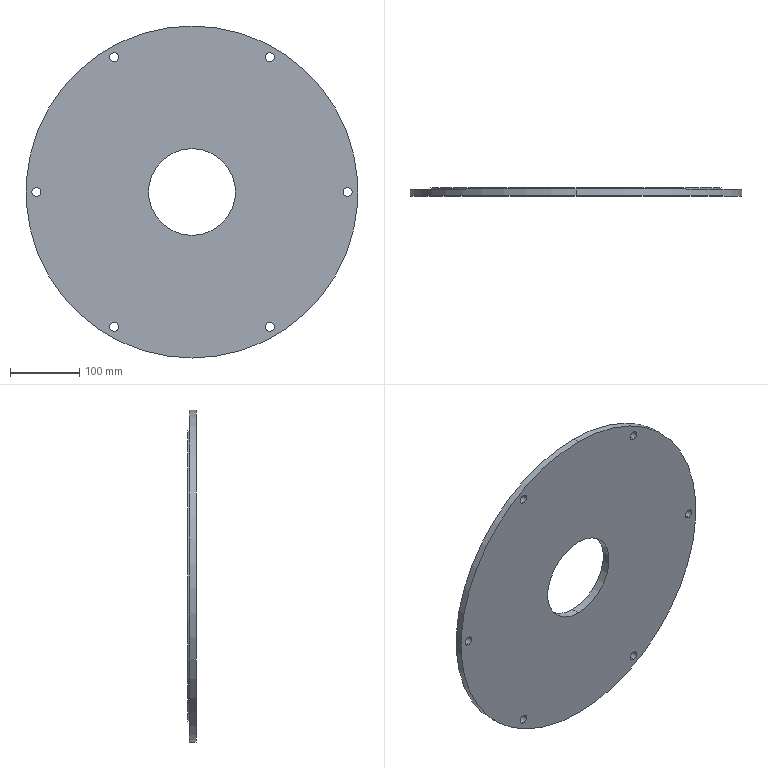Part | SolidWorks | features Extrusion 1, HoleWzd 1, ICE 1 | 1 solid | 21 faces | box 480 x 12 x 480 mm | volume 1930239 mm3 | cylinder 18 | plane 3 | commonest cylinder face diameters 13 x12 125.5 x2 420 x2 480 x2
STEP:
#1=CARTESIAN_POINT('',(0.,4.,210.));
#2=VERTEX_POINT('',#1);
#3=CARTESIAN_POINT('',(0.,4.,-210.));
#4=VERTEX_POINT('',#3);
#5=CARTESIAN_POINT('',(0.,4.,0.));
#6=DIRECTION('',(0.,1.,0.));
#7=DIRECTION('',(0.,0.,1.));
#8=AXIS2_PLACEMENT_3D('',#5,#6,#7);
#9=CIRCLE('',#8,210.);
#10=EDGE_CURVE('',#2,#4,#9,.T.);
#11=ORIENTED_EDGE('',*,*,#10,.T.);
#12=CARTESIAN_POINT('',(0.,6.,-210.));
#13=VERTEX_POINT('',#12);
#14=CARTESIAN_POINT('',(0.,4.,-210.));
#15=DIRECTION('',(0.,1.,0.));
#16=VECTOR('',#15,1000.);
#17=LINE('',#14,#16);
#18=EDGE_CURVE('',#4,#13,#17,.T.);
#19=ORIENTED_EDGE('',*,*,#18,.T.);
#20=CARTESIAN_POINT('',(0.,6.,210.));
#21=VERTEX_POINT('',#20);
#22=CARTESIAN_POINT('',(0.,6.,0.));
#23=DIRECTION('',(0.,1.,0.));
#24=DIRECTION('',(0.,0.,1.));
#25=AXIS2_PLACEMENT_3D('',#22,#23,#24);
#26=CIRCLE('',#25,210.);
#27=EDGE_CURVE('',#21,#13,#26,.T.);
#28=ORIENTED_EDGE('',*,*,#27,.F.);
#29=CARTESIAN_POINT('',(0.,4.,210.));
#30=DIRECTION('',(0.,1.,0.));
#31=VECTOR('',#30,1000.);
#32=LINE('',#29,#31);
#33=EDGE_CURVE('',#2,#21,#32,.T.);
#34=ORIENTED_EDGE('',*,*,#33,.F.);
#35=EDGE_LOOP('',(#11,#19,#28,#34));
#36=FACE_OUTER_BOUND('',#35,.T.);
#37=CARTESIAN_POINT('',(0.,4.,0.));
#38=DIRECTION('',(0.,1.,0.));
#39=DIRECTION('',(0.,0.,1.));
#40=AXIS2_PLACEMENT_3D('',#37,#38,#39);
#41=CYLINDRICAL_SURFACE('',#40,210.);
#42=ADVANCED_FACE('',(#36),#41,.T.);
#43=CARTESIAN_POINT('',(0.,6.,-62.75));
#44=VERTEX_POINT('',#43);
#45=CARTESIAN_POINT('',(0.,6.,62.75));
#46=VERTEX_POINT('',#45);
#47=CARTESIAN_POINT('',(0.,6.,0.));
#48=DIRECTION('',(0.,1.,0.));
#49=DIRECTION('',(0.,0.,1.));
#50=AXIS2_PLACEMENT_3D('',#47,#48,#49);
#51=CIRCLE('',#50,62.75);
#52=EDGE_CURVE('',#44,#46,#51,.T.);
#53=ORIENTED_EDGE('',*,*,#52,.T.);
#54=CARTESIAN_POINT('',(0.,-6.,62.75));
#55=VERTEX_POINT('',#54);
#56=CARTESIAN_POINT('',(0.,6.,62.75));
#57=DIRECTION('',(0.,-1.,0.));
#58=VECTOR('',#57,1000.);
#59=LINE('',#56,#58);
#60=EDGE_CURVE('',#46,#55,#59,.T.);
#61=ORIENTED_EDGE('',*,*,#60,.T.);
#62=CARTESIAN_POINT('',(0.,-6.,-62.75));
#63=VERTEX_POINT('',#62);
#64=CARTESIAN_POINT('',(0.,-6.,0.));
#65=DIRECTION('',(0.,1.,0.));
#66=DIRECTION('',(0.,0.,1.));
#67=AXIS2_PLACEMENT_3D('',#64,#65,#66);
#68=CIRCLE('',#67,62.75);
#69=EDGE_CURVE('',#63,#55,#68,.T.);
#70=ORIENTED_EDGE('',*,*,#69,.F.);
#71=CARTESIAN_POINT('',(0.,6.,-62.75));
#72=DIRECTION('',(0.,-1.,0.));
#73=VECTOR('',#72,1000.);
#74=LINE('',#71,#73);
#75=EDGE_CURVE('',#44,#63,#74,.T.);
#76=ORIENTED_EDGE('',*,*,#75,.F.);
#77=EDGE_LOOP('',(#53,#61,#70,#76));
#78=FACE_OUTER_BOUND('',#77,.T.);
#79=CARTESIAN_POINT('',(0.,6.,0.));
#80=DIRECTION('',(0.,-1.,0.));
#81=DIRECTION('',(0.,0.,-1.));
#82=AXIS2_PLACEMENT_3D('',#79,#80,#81);
#83=CYLINDRICAL_SURFACE('',#82,62.75);
#84=ADVANCED_FACE('',(#78),#83,.F.);
#85=CARTESIAN_POINT('',(112.5,-6.,188.356));
#86=VERTEX_POINT('',#85);
#87=CARTESIAN_POINT('',(112.5,-6.,201.356));
#88=VERTEX_POINT('',#87);
#89=CARTESIAN_POINT('',(112.5,-6.,194.856));
#90=DIRECTION('',(0.,1.,0.));
#91=DIRECTION('',(0.,0.,1.));
#92=AXIS2_PLACEMENT_3D('',#89,#90,#91);
#93=CIRCLE('',#92,6.5);
#94=EDGE_CURVE('',#86,#88,#93,.T.);
#95=ORIENTED_EDGE('',*,*,#94,.F.);
#96=CARTESIAN_POINT('',(112.5,4.,188.356));
#97=VERTEX_POINT('',#96);
#98=CARTESIAN_POINT('',(112.5,6.,188.356));
#99=DIRECTION('',(0.,1.,0.));
#100=VECTOR('',#99,1000.);
#101=LINE('',#98,#100);
#102=EDGE_CURVE('',#86,#97,#101,.T.);
#103=ORIENTED_EDGE('',*,*,#102,.T.);
#104=CARTESIAN_POINT('',(112.5,4.,201.356));
#105=VERTEX_POINT('',#104);
#106=CARTESIAN_POINT('',(112.5,4.,194.856));
#107=DIRECTION('',(0.,-1.,0.));
#108=DIRECTION('',(0.,0.,1.));
#109=AXIS2_PLACEMENT_3D('',#106,#107,#108);
#110=CIRCLE('',#109,6.5);
#111=EDGE_CURVE('',#105,#97,#110,.T.);
#112=ORIENTED_EDGE('',*,*,#111,.F.);
#113=CARTESIAN_POINT('',(112.5,6.,201.356));
#114=DIRECTION('',(0.,1.,0.));
#115=VECTOR('',#114,1000.);
#116=LINE('',#113,#115);
#117=EDGE_CURVE('',#88,#105,#116,.T.);
#118=ORIENTED_EDGE('',*,*,#117,.F.);
#119=EDGE_LOOP('',(#95,#103,#112,#118));
#120=FACE_OUTER_BOUND('',#119,.T.);
#121=CARTESIAN_POINT('',(112.5,6.,194.856));
#122=DIRECTION('',(0.,1.,0.));
#123=DIRECTION('',(0.,0.,1.));
#124=AXIS2_PLACEMENT_3D('',#121,#122,#123);
#125=CYLINDRICAL_SURFACE('',#124,6.5);
#126=ADVANCED_FACE('',(#120),#125,.F.);
#127=CARTESIAN_POINT('',(-112.5,-6.,188.356));
#128=VERTEX_POINT('',#127);
#129=CARTESIAN_POINT('',(-112.5,-6.,201.356));
#130=VERTEX_POINT('',#129);
#131=CARTESIAN_POINT('',(-112.5,-6.,194.856));
#132=DIRECTION('',(0.,1.,0.));
#133=DIRECTION('',(0.,0.,1.));
#134=AXIS2_PLACEMENT_3D('',#131,#132,#133);
#135=CIRCLE('',#134,6.5);
#136=EDGE_CURVE('',#128,#130,#135,.T.);
#137=ORIENTED_EDGE('',*,*,#136,.F.);
#138=CARTESIAN_POINT('',(-112.5,4.,188.356));
#139=VERTEX_POINT('',#138);
#140=CARTESIAN_POINT('',(-112.5,6.,188.356));
#141=DIRECTION('',(0.,1.,0.));
#142=VECTOR('',#141,1000.);
#143=LINE('',#140,#142);
#144=EDGE_CURVE('',#128,#139,#143,.T.);
#145=ORIENTED_EDGE('',*,*,#144,.T.);
#146=CARTESIAN_POINT('',(-112.5,4.,201.356));
#147=VERTEX_POINT('',#146);
#148=CARTESIAN_POINT('',(-112.5,4.,194.856));
#149=DIRECTION('',(0.,-1.,0.));
#150=DIRECTION('',(0.,0.,1.));
#151=AXIS2_PLACEMENT_3D('',#148,#149,#150);
#152=CIRCLE('',#151,6.5);
#153=EDGE_CURVE('',#147,#139,#152,.T.);
#154=ORIENTED_EDGE('',*,*,#153,.F.);
#155=CARTESIAN_POINT('',(-112.5,6.,201.356));
#156=DIRECTION('',(0.,1.,0.));
#157=VECTOR('',#156,1000.);
#158=LINE('',#155,#157);
#159=EDGE_CURVE('',#130,#147,#158,.T.);
#160=ORIENTED_EDGE('',*,*,#159,.F.);
#161=EDGE_LOOP('',(#137,#145,#154,#160));
#162=FACE_OUTER_BOUND('',#161,.T.);
#163=CARTESIAN_POINT('',(-112.5,6.,194.856));
#164=DIRECTION('',(0.,1.,0.));
#165=DIRECTION('',(0.,0.,1.));
#166=AXIS2_PLACEMENT_3D('',#163,#164,#165);
#167=CYLINDRICAL_SURFACE('',#166,6.5);
#168=ADVANCED_FACE('',(#162),#167,.F.);
#169=CARTESIAN_POINT('',(-225.,-6.,-6.5));
#170=VERTEX_POINT('',#169);
#171=CARTESIAN_POINT('',(-225.,-6.,6.5));
#172=VERTEX_POINT('',#171);
#173=CARTESIAN_POINT('',(-225.,-6.,0.));
#174=DIRECTION('',(0.,1.,0.));
#175=DIRECTION('',(0.,0.,1.));
#176=AXIS2_PLACEMENT_3D('',#173,#174,#175);
#177=CIRCLE('',#176,6.5);
#178=EDGE_CURVE('',#170,#172,#177,.T.);
#179=ORIENTED_EDGE('',*,*,#178,.F.);
#180=CARTESIAN_POINT('',(-225.,4.,-6.5));
#181=VERTEX_POINT('',#180);
#182=CARTESIAN_POINT('',(-225.,6.,-6.5));
#183=DIRECTION('',(0.,1.,0.));
#184=VECTOR('',#183,1000.);
#185=LINE('',#182,#184);
#186=EDGE_CURVE('',#170,#181,#185,.T.);
#187=ORIENTED_EDGE('',*,*,#186,.T.);
#188=CARTESIAN_POINT('',(-225.,4.,6.5));
#189=VERTEX_POINT('',#188);
#190=CARTESIAN_POINT('',(-225.,4.,0.));
#191=DIRECTION('',(0.,-1.,0.));
#192=DIRECTION('',(0.,0.,1.));
#193=AXIS2_PLACEMENT_3D('',#190,#191,#192);
#194=CIRCLE('',#193,6.5);
#195=EDGE_CURVE('',#189,#181,#194,.T.);
#196=ORIENTED_EDGE('',*,*,#195,.F.);
#197=CARTESIAN_POINT('',(-225.,6.,6.5));
#198=DIRECTION('',(0.,1.,0.));
#199=VECTOR('',#198,1000.);
#200=LINE('',#197,#199);
#201=EDGE_CURVE('',#172,#189,#200,.T.);
#202=ORIENTED_EDGE('',*,*,#201,.F.);
#203=EDGE_LOOP('',(#179,#187,#196,#202));
#204=FACE_OUTER_BOUND('',#203,.T.);
#205=CARTESIAN_POINT('',(-225.,6.,0.));
#206=DIRECTION('',(0.,1.,0.));
#207=DIRECTION('',(0.,0.,1.));
#208=AXIS2_PLACEMENT_3D('',#205,#206,#207);
#209=CYLINDRICAL_SURFACE('',#208,6.5);
#210=ADVANCED_FACE('',(#204),#209,.F.);
#211=CARTESIAN_POINT('',(-112.5,-6.,-201.356));
#212=VERTEX_POINT('',#211);
#213=CARTESIAN_POINT('',(-112.5,-6.,-188.356));
#214=VERTEX_POINT('',#213);
#215=CARTESIAN_POINT('',(-112.5,-6.,-194.856));
#216=DIRECTION('',(0.,1.,0.));
#217=DIRECTION('',(0.,0.,1.));
#218=AXIS2_PLACEMENT_3D('',#215,#216,#217);
#219=CIRCLE('',#218,6.5);
#220=EDGE_CURVE('',#212,#214,#219,.T.);
#221=ORIENTED_EDGE('',*,*,#220,.F.);
#222=CARTESIAN_POINT('',(-112.5,4.,-201.356));
#223=VERTEX_POINT('',#222);
#224=CARTESIAN_POINT('',(-112.5,6.,-201.356));
#225=DIRECTION('',(0.,1.,0.));
#226=VECTOR('',#225,1000.);
#227=LINE('',#224,#226);
#228=EDGE_CURVE('',#212,#223,#227,.T.);
#229=ORIENTED_EDGE('',*,*,#228,.T.);
#230=CARTESIAN_POINT('',(-112.5,4.,-188.356));
#231=VERTEX_POINT('',#230);
#232=CARTESIAN_POINT('',(-112.5,4.,-194.856));
#233=DIRECTION('',(0.,-1.,0.));
#234=DIRECTION('',(0.,0.,1.));
#235=AXIS2_PLACEMENT_3D('',#232,#233,#234);
#236=CIRCLE('',#235,6.5);
#237=EDGE_CURVE('',#231,#223,#236,.T.);
#238=ORIENTED_EDGE('',*,*,#237,.F.);
#239=CARTESIAN_POINT('',(-112.5,6.,-188.356));
#240=DIRECTION('',(0.,1.,0.));
#241=VECTOR('',#240,1000.);
#242=LINE('',#239,#241);
#243=EDGE_CURVE('',#214,#231,#242,.T.);
#244=ORIENTED_EDGE('',*,*,#243,.F.);
#245=EDGE_LOOP('',(#221,#229,#238,#244));
#246=FACE_OUTER_BOUND('',#245,.T.);
#247=CARTESIAN_POINT('',(-112.5,6.,-194.856));
#248=DIRECTION('',(0.,1.,0.));
#249=DIRECTION('',(0.,0.,1.));
#250=AXIS2_PLACEMENT_3D('',#247,#248,#249);
#251=CYLINDRICAL_SURFACE('',#250,6.5);
#252=ADVANCED_FACE('',(#246),#251,.F.);
#253=CARTESIAN_POINT('',(112.5,-6.,-201.356));
#254=VERTEX_POINT('',#253);
#255=CARTESIAN_POINT('',(112.5,-6.,-188.356));
#256=VERTEX_POINT('',#255);
#257=CARTESIAN_POINT('',(112.5,-6.,-194.856));
#258=DIRECTION('',(0.,1.,0.));
#259=DIRECTION('',(0.,0.,1.));
#260=AXIS2_PLACEMENT_3D('',#257,#258,#259);
#261=CIRCLE('',#260,6.5);
#262=EDGE_CURVE('',#254,#256,#261,.T.);
#263=ORIENTED_EDGE('',*,*,#262,.F.);
#264=CARTESIAN_POINT('',(112.5,4.,-201.356));
#265=VERTEX_POINT('',#264);
#266=CARTESIAN_POINT('',(112.5,6.,-201.356));
#267=DIRECTION('',(0.,1.,0.));
#268=VECTOR('',#267,1000.);
#269=LINE('',#266,#268);
#270=EDGE_CURVE('',#254,#265,#269,.T.);
#271=ORIENTED_EDGE('',*,*,#270,.T.);
#272=CARTESIAN_POINT('',(112.5,4.,-188.356));
#273=VERTEX_POINT('',#272);
#274=CARTESIAN_POINT('',(112.5,4.,-194.856));
#275=DIRECTION('',(0.,-1.,0.));
#276=DIRECTION('',(0.,0.,1.));
#277=AXIS2_PLACEMENT_3D('',#274,#275,#276);
#278=CIRCLE('',#277,6.5);
#279=EDGE_CURVE('',#273,#265,#278,.T.);
#280=ORIENTED_EDGE('',*,*,#279,.F.);
#281=CARTESIAN_POINT('',(112.5,6.,-188.356));
#282=DIRECTION('',(0.,1.,0.));
#283=VECTOR('',#282,1000.);
#284=LINE('',#281,#283);
#285=EDGE_CURVE('',#256,#273,#284,.T.);
#286=ORIENTED_EDGE('',*,*,#285,.F.);
#287=EDGE_LOOP('',(#263,#271,#280,#286));
#288=FACE_OUTER_BOUND('',#287,.T.);
#289=CARTESIAN_POINT('',(112.5,6.,-194.856));
#290=DIRECTION('',(0.,1.,0.));
#291=DIRECTION('',(0.,0.,1.));
#292=AXIS2_PLACEMENT_3D('',#289,#290,#291);
#293=CYLINDRICAL_SURFACE('',#292,6.5);
#294=ADVANCED_FACE('',(#288),#293,.F.);
#295=CARTESIAN_POINT('',(225.,-6.,-6.5));
#296=VERTEX_POINT('',#295);
#297=CARTESIAN_POINT('',(225.,-6.,6.5));
#298=VERTEX_POINT('',#297);
#299=CARTESIAN_POINT('',(225.,-6.,0.));
#300=DIRECTION('',(0.,1.,0.));
#301=DIRECTION('',(0.,0.,1.));
#302=AXIS2_PLACEMENT_3D('',#299,#300,#301);
#303=CIRCLE('',#302,6.5);
#304=EDGE_CURVE('',#296,#298,#303,.T.);
#305=ORIENTED_EDGE('',*,*,#304,.F.);
#306=CARTESIAN_POINT('',(225.,4.,-6.5));
#307=VERTEX_POINT('',#306);
#308=CARTESIAN_POINT('',(225.,6.,-6.5));
#309=DIRECTION('',(0.,1.,0.));
#310=VECTOR('',#309,1000.);
#311=LINE('',#308,#310);
#312=EDGE_CURVE('',#296,#307,#311,.T.);
#313=ORIENTED_EDGE('',*,*,#312,.T.);
#314=CARTESIAN_POINT('',(225.,4.,6.5));
#315=VERTEX_POINT('',#314);
#316=CARTESIAN_POINT('',(225.,4.,0.));
#317=DIRECTION('',(0.,-1.,0.));
#318=DIRECTION('',(0.,0.,1.));
#319=AXIS2_PLACEMENT_3D('',#316,#317,#318);
#320=CIRCLE('',#319,6.5);
#321=EDGE_CURVE('',#315,#307,#320,.T.);
#322=ORIENTED_EDGE('',*,*,#321,.F.);
#323=CARTESIAN_POINT('',(225.,6.,6.5));
#324=DIRECTION('',(0.,1.,0.));
#325=VECTOR('',#324,1000.);
#326=LINE('',#323,#325);
#327=EDGE_CURVE('',#298,#315,#326,.T.);
#328=ORIENTED_EDGE('',*,*,#327,.F.);
#329=EDGE_LOOP('',(#305,#313,#322,#328));
#330=FACE_OUTER_BOUND('',#329,.T.);
#331=CARTESIAN_POINT('',(225.,6.,0.));
#332=DIRECTION('',(0.,1.,0.));
#333=DIRECTION('',(0.,0.,1.));
#334=AXIS2_PLACEMENT_3D('',#331,#332,#333);
#335=CYLINDRICAL_SURFACE('',#334,6.5);
#336=ADVANCED_FACE('',(#330),#335,.F.);
#337=CARTESIAN_POINT('',(0.,4.,240.));
#338=VERTEX_POINT('',#337);
#339=CARTESIAN_POINT('',(0.,4.,-240.));
#340=VERTEX_POINT('',#339);
#341=CARTESIAN_POINT('',(0.,4.,0.));
#342=DIRECTION('',(0.,1.,0.));
#343=DIRECTION('',(0.,0.,1.));
#344=AXIS2_PLACEMENT_3D('',#341,#342,#343);
#345=CIRCLE('',#344,240.);
#346=EDGE_CURVE('',#338,#340,#345,.T.);
#347=ORIENTED_EDGE('',*,*,#346,.F.);
#348=CARTESIAN_POINT('',(0.,-6.,240.));
#349=VERTEX_POINT('',#348);
#350=CARTESIAN_POINT('',(0.,6.,240.));
#351=DIRECTION('',(0.,-1.,0.));
#352=VECTOR('',#351,1000.);
#353=LINE('',#350,#352);
#354=EDGE_CURVE('',#338,#349,#353,.T.);
#355=ORIENTED_EDGE('',*,*,#354,.T.);
#356=CARTESIAN_POINT('',(0.,-6.,-240.));
#357=VERTEX_POINT('',#356);
#358=CARTESIAN_POINT('',(0.,-6.,0.));
#359=DIRECTION('',(0.,1.,0.));
#360=DIRECTION('',(0.,0.,1.));
#361=AXIS2_PLACEMENT_3D('',#358,#359,#360);
#362=CIRCLE('',#361,240.);
#363=EDGE_CURVE('',#349,#357,#362,.T.);
#364=ORIENTED_EDGE('',*,*,#363,.T.);
#365=CARTESIAN_POINT('',(0.,6.,-240.));
#366=DIRECTION('',(0.,-1.,0.));
#367=VECTOR('',#366,1000.);
#368=LINE('',#365,#367);
#369=EDGE_CURVE('',#340,#357,#368,.T.);
#370=ORIENTED_EDGE('',*,*,#369,.F.);
#371=EDGE_LOOP('',(#347,#355,#364,#370));
#372=FACE_OUTER_BOUND('',#371,.T.);
#373=CARTESIAN_POINT('',(0.,6.,0.));
#374=DIRECTION('',(0.,-1.,0.));
#375=DIRECTION('',(0.,0.,-1.));
#376=AXIS2_PLACEMENT_3D('',#373,#374,#375);
#377=CYLINDRICAL_SURFACE('',#376,240.);
#378=ADVANCED_FACE('',(#372),#377,.T.);
#379=ORIENTED_EDGE('',*,*,#52,.F.);
#380=CARTESIAN_POINT('',(0.,6.,0.));
#381=DIRECTION('',(0.,1.,0.));
#382=DIRECTION('',(0.,0.,1.));
#383=AXIS2_PLACEMENT_3D('',#380,#381,#382);
#384=CIRCLE('',#383,62.75);
#385=EDGE_CURVE('',#46,#44,#384,.T.);
#386=ORIENTED_EDGE('',*,*,#385,.F.);
#387=EDGE_LOOP('',(#379,#386));
#388=FACE_BOUND('',#387,.T.);
#389=ORIENTED_EDGE('',*,*,#27,.T.);
#390=CARTESIAN_POINT('',(0.,6.,0.));
#391=DIRECTION('',(0.,1.,0.));
#392=DIRECTION('',(0.,0.,1.));
#393=AXIS2_PLACEMENT_3D('',#390,#391,#392);
#394=CIRCLE('',#393,210.);
#395=EDGE_CURVE('',#13,#21,#394,.T.);
#396=ORIENTED_EDGE('',*,*,#395,.T.);
#397=EDGE_LOOP('',(#389,#396));
#398=FACE_OUTER_BOUND('',#397,.T.);
#399=CARTESIAN_POINT('',(0.,6.,0.));
#400=DIRECTION('',(0.,1.,0.));
#401=DIRECTION('',(0.,0.,1.));
#402=AXIS2_PLACEMENT_3D('',#399,#400,#401);
#403=PLANE('',#402);
#404=ADVANCED_FACE('',(#388,#398),#403,.T.);
#405=ORIENTED_EDGE('',*,*,#354,.F.);
#406=CARTESIAN_POINT('',(0.,4.,0.));
#407=DIRECTION('',(0.,1.,0.));
#408=DIRECTION('',(0.,0.,1.));
#409=AXIS2_PLACEMENT_3D('',#406,#407,#408);
#410=CIRCLE('',#409,240.);
#411=EDGE_CURVE('',#340,#338,#410,.T.);
#412=ORIENTED_EDGE('',*,*,#411,.F.);
#413=ORIENTED_EDGE('',*,*,#369,.T.);
#414=CARTESIAN_POINT('',(0.,-6.,0.));
#415=DIRECTION('',(0.,1.,0.));
#416=DIRECTION('',(0.,0.,1.));
#417=AXIS2_PLACEMENT_3D('',#414,#415,#416);
#418=CIRCLE('',#417,240.);
#419=EDGE_CURVE('',#357,#349,#418,.T.);
#420=ORIENTED_EDGE('',*,*,#419,.T.);
#421=EDGE_LOOP('',(#405,#412,#413,#420));
#422=FACE_OUTER_BOUND('',#421,.T.);
#423=CARTESIAN_POINT('',(0.,6.,0.));
#424=DIRECTION('',(0.,-1.,0.));
#425=DIRECTION('',(0.,0.,-1.));
#426=AXIS2_PLACEMENT_3D('',#423,#424,#425);
#427=CYLINDRICAL_SURFACE('',#426,240.);
#428=ADVANCED_FACE('',(#422),#427,.T.);
#429=ORIENTED_EDGE('',*,*,#312,.F.);
#430=CARTESIAN_POINT('',(225.,-6.,0.));
#431=DIRECTION('',(0.,1.,0.));
#432=DIRECTION('',(0.,0.,1.));
#433=AXIS2_PLACEMENT_3D('',#430,#431,#432);
#434=CIRCLE('',#433,6.5);
#435=EDGE_CURVE('',#298,#296,#434,.T.);
#436=ORIENTED_EDGE('',*,*,#435,.F.);
#437=ORIENTED_EDGE('',*,*,#327,.T.);
#438=CARTESIAN_POINT('',(225.,4.,0.));
#439=DIRECTION('',(0.,-1.,0.));
#440=DIRECTION('',(0.,0.,1.));
#441=AXIS2_PLACEMENT_3D('',#438,#439,#440);
#442=CIRCLE('',#441,6.5);
#443=EDGE_CURVE('',#307,#315,#442,.T.);
#444=ORIENTED_EDGE('',*,*,#443,.F.);
#445=EDGE_LOOP('',(#429,#436,#437,#444));
#446=FACE_OUTER_BOUND('',#445,.T.);
#447=CARTESIAN_POINT('',(225.,6.,0.));
#448=DIRECTION('',(0.,1.,0.));
#449=DIRECTION('',(0.,0.,1.));
#450=AXIS2_PLACEMENT_3D('',#447,#448,#449);
#451=CYLINDRICAL_SURFACE('',#450,6.5);
#452=ADVANCED_FACE('',(#446),#451,.F.);
#453=ORIENTED_EDGE('',*,*,#270,.F.);
#454=CARTESIAN_POINT('',(112.5,-6.,-194.856));
#455=DIRECTION('',(0.,1.,0.));
#456=DIRECTION('',(0.,0.,1.));
#457=AXIS2_PLACEMENT_3D('',#454,#455,#456);
#458=CIRCLE('',#457,6.5);
#459=EDGE_CURVE('',#256,#254,#458,.T.);
#460=ORIENTED_EDGE('',*,*,#459,.F.);
#461=ORIENTED_EDGE('',*,*,#285,.T.);
#462=CARTESIAN_POINT('',(112.5,4.,-194.856));
#463=DIRECTION('',(0.,-1.,0.));
#464=DIRECTION('',(0.,0.,1.));
#465=AXIS2_PLACEMENT_3D('',#462,#463,#464);
#466=CIRCLE('',#465,6.5);
#467=EDGE_CURVE('',#265,#273,#466,.T.);
#468=ORIENTED_EDGE('',*,*,#467,.F.);
#469=EDGE_LOOP('',(#453,#460,#461,#468));
#470=FACE_OUTER_BOUND('',#469,.T.);
#471=CARTESIAN_POINT('',(112.5,6.,-194.856));
#472=DIRECTION('',(0.,1.,0.));
#473=DIRECTION('',(0.,0.,1.));
#474=AXIS2_PLACEMENT_3D('',#471,#472,#473);
#475=CYLINDRICAL_SURFACE('',#474,6.5);
#476=ADVANCED_FACE('',(#470),#475,.F.);
#477=ORIENTED_EDGE('',*,*,#228,.F.);
#478=CARTESIAN_POINT('',(-112.5,-6.,-194.856));
#479=DIRECTION('',(0.,1.,0.));
#480=DIRECTION('',(0.,0.,1.));
#481=AXIS2_PLACEMENT_3D('',#478,#479,#480);
#482=CIRCLE('',#481,6.5);
#483=EDGE_CURVE('',#214,#212,#482,.T.);
#484=ORIENTED_EDGE('',*,*,#483,.F.);
#485=ORIENTED_EDGE('',*,*,#243,.T.);
#486=CARTESIAN_POINT('',(-112.5,4.,-194.856));
#487=DIRECTION('',(0.,-1.,0.));
#488=DIRECTION('',(0.,0.,1.));
#489=AXIS2_PLACEMENT_3D('',#486,#487,#488);
#490=CIRCLE('',#489,6.5);
#491=EDGE_CURVE('',#223,#231,#490,.T.);
#492=ORIENTED_EDGE('',*,*,#491,.F.);
#493=EDGE_LOOP('',(#477,#484,#485,#492));
#494=FACE_OUTER_BOUND('',#493,.T.);
#495=CARTESIAN_POINT('',(-112.5,6.,-194.856));
#496=DIRECTION('',(0.,1.,0.));
#497=DIRECTION('',(0.,0.,1.));
#498=AXIS2_PLACEMENT_3D('',#495,#496,#497);
#499=CYLINDRICAL_SURFACE('',#498,6.5);
#500=ADVANCED_FACE('',(#494),#499,.F.);
#501=ORIENTED_EDGE('',*,*,#186,.F.);
#502=CARTESIAN_POINT('',(-225.,-6.,0.));
#503=DIRECTION('',(0.,1.,0.));
#504=DIRECTION('',(0.,0.,1.));
#505=AXIS2_PLACEMENT_3D('',#502,#503,#504);
#506=CIRCLE('',#505,6.5);
#507=EDGE_CURVE('',#172,#170,#506,.T.);
#508=ORIENTED_EDGE('',*,*,#507,.F.);
#509=ORIENTED_EDGE('',*,*,#201,.T.);
#510=CARTESIAN_POINT('',(-225.,4.,0.));
#511=DIRECTION('',(0.,-1.,0.));
#512=DIRECTION('',(0.,0.,1.));
#513=AXIS2_PLACEMENT_3D('',#510,#511,#512);
#514=CIRCLE('',#513,6.5);
#515=EDGE_CURVE('',#181,#189,#514,.T.);
#516=ORIENTED_EDGE('',*,*,#515,.F.);
#517=EDGE_LOOP('',(#501,#508,#509,#516));
#518=FACE_OUTER_BOUND('',#517,.T.);
#519=CARTESIAN_POINT('',(-225.,6.,0.));
#520=DIRECTION('',(0.,1.,0.));
#521=DIRECTION('',(0.,0.,1.));
#522=AXIS2_PLACEMENT_3D('',#519,#520,#521);
#523=CYLINDRICAL_SURFACE('',#522,6.5);
#524=ADVANCED_FACE('',(#518),#523,.F.);
#525=ORIENTED_EDGE('',*,*,#144,.F.);
#526=CARTESIAN_POINT('',(-112.5,-6.,194.856));
#527=DIRECTION('',(0.,1.,0.));
#528=DIRECTION('',(0.,0.,1.));
#529=AXIS2_PLACEMENT_3D('',#526,#527,#528);
#530=CIRCLE('',#529,6.5);
#531=EDGE_CURVE('',#130,#128,#530,.T.);
#532=ORIENTED_EDGE('',*,*,#531,.F.);
#533=ORIENTED_EDGE('',*,*,#159,.T.);
#534=CARTESIAN_POINT('',(-112.5,4.,194.856));
#535=DIRECTION('',(0.,-1.,0.));
#536=DIRECTION('',(0.,0.,1.));
#537=AXIS2_PLACEMENT_3D('',#534,#535,#536);
#538=CIRCLE('',#537,6.5);
#539=EDGE_CURVE('',#139,#147,#538,.T.);
#540=ORIENTED_EDGE('',*,*,#539,.F.);
#541=EDGE_LOOP('',(#525,#532,#533,#540));
#542=FACE_OUTER_BOUND('',#541,.T.);
#543=CARTESIAN_POINT('',(-112.5,6.,194.856));
#544=DIRECTION('',(0.,1.,0.));
#545=DIRECTION('',(0.,0.,1.));
#546=AXIS2_PLACEMENT_3D('',#543,#544,#545);
#547=CYLINDRICAL_SURFACE('',#546,6.5);
#548=ADVANCED_FACE('',(#542),#547,.F.);
#549=ORIENTED_EDGE('',*,*,#102,.F.);
#550=CARTESIAN_POINT('',(112.5,-6.,194.856));
#551=DIRECTION('',(0.,1.,0.));
#552=DIRECTION('',(0.,0.,1.));
#553=AXIS2_PLACEMENT_3D('',#550,#551,#552);
#554=CIRCLE('',#553,6.5);
#555=EDGE_CURVE('',#88,#86,#554,.T.);
#556=ORIENTED_EDGE('',*,*,#555,.F.);
#557=ORIENTED_EDGE('',*,*,#117,.T.);
#558=CARTESIAN_POINT('',(112.5,4.,194.856));
#559=DIRECTION('',(0.,-1.,0.));
#560=DIRECTION('',(0.,0.,1.));
#561=AXIS2_PLACEMENT_3D('',#558,#559,#560);
#562=CIRCLE('',#561,6.5);
#563=EDGE_CURVE('',#97,#105,#562,.T.);
#564=ORIENTED_EDGE('',*,*,#563,.F.);
#565=EDGE_LOOP('',(#549,#556,#557,#564));
#566=FACE_OUTER_BOUND('',#565,.T.);
#567=CARTESIAN_POINT('',(112.5,6.,194.856));
#568=DIRECTION('',(0.,1.,0.));
#569=DIRECTION('',(0.,0.,1.));
#570=AXIS2_PLACEMENT_3D('',#567,#568,#569);
#571=CYLINDRICAL_SURFACE('',#570,6.5);
#572=ADVANCED_FACE('',(#566),#571,.F.);
#573=ORIENTED_EDGE('',*,*,#555,.T.);
#574=ORIENTED_EDGE('',*,*,#94,.T.);
#575=EDGE_LOOP('',(#573,#574));
#576=FACE_BOUND('',#575,.T.);
#577=ORIENTED_EDGE('',*,*,#531,.T.);
#578=ORIENTED_EDGE('',*,*,#136,.T.);
#579=EDGE_LOOP('',(#577,#578));
#580=FACE_BOUND('',#579,.T.);
#581=ORIENTED_EDGE('',*,*,#507,.T.);
#582=ORIENTED_EDGE('',*,*,#178,.T.);
#583=EDGE_LOOP('',(#581,#582));
#584=FACE_BOUND('',#583,.T.);
#585=ORIENTED_EDGE('',*,*,#483,.T.);
#586=ORIENTED_EDGE('',*,*,#220,.T.);
#587=EDGE_LOOP('',(#585,#586));
#588=FACE_BOUND('',#587,.T.);
#589=ORIENTED_EDGE('',*,*,#459,.T.);
#590=ORIENTED_EDGE('',*,*,#262,.T.);
#591=EDGE_LOOP('',(#589,#590));
#592=FACE_BOUND('',#591,.T.);
#593=ORIENTED_EDGE('',*,*,#435,.T.);
#594=ORIENTED_EDGE('',*,*,#304,.T.);
#595=EDGE_LOOP('',(#593,#594));
#596=FACE_BOUND('',#595,.T.);
#597=ORIENTED_EDGE('',*,*,#419,.F.);
#598=ORIENTED_EDGE('',*,*,#363,.F.);
#599=EDGE_LOOP('',(#597,#598));
#600=FACE_OUTER_BOUND('',#599,.T.);
#601=ORIENTED_EDGE('',*,*,#69,.T.);
#602=CARTESIAN_POINT('',(0.,-6.,0.));
#603=DIRECTION('',(0.,1.,0.));
#604=DIRECTION('',(0.,0.,1.));
#605=AXIS2_PLACEMENT_3D('',#602,#603,#604);
#606=CIRCLE('',#605,62.75);
#607=EDGE_CURVE('',#55,#63,#606,.T.);
#608=ORIENTED_EDGE('',*,*,#607,.T.);
#609=EDGE_LOOP('',(#601,#608));
#610=FACE_BOUND('',#609,.T.);
#611=CARTESIAN_POINT('',(0.,-6.,0.));
#612=DIRECTION('',(0.,1.,0.));
#613=DIRECTION('',(0.,0.,1.));
#614=AXIS2_PLACEMENT_3D('',#611,#612,#613);
#615=PLANE('',#614);
#616=ADVANCED_FACE('',(#576,#580,#584,#588,#592,#596,#600,#610),#615,.F.);
#617=ORIENTED_EDGE('',*,*,#60,.F.);
#618=ORIENTED_EDGE('',*,*,#385,.T.);
#619=ORIENTED_EDGE('',*,*,#75,.T.);
#620=ORIENTED_EDGE('',*,*,#607,.F.);
#621=EDGE_LOOP('',(#617,#618,#619,#620));
#622=FACE_OUTER_BOUND('',#621,.T.);
#623=CARTESIAN_POINT('',(0.,6.,0.));
#624=DIRECTION('',(0.,-1.,0.));
#625=DIRECTION('',(0.,0.,-1.));
#626=AXIS2_PLACEMENT_3D('',#623,#624,#625);
#627=CYLINDRICAL_SURFACE('',#626,62.75);
#628=ADVANCED_FACE('',(#622),#627,.F.);
#629=ORIENTED_EDGE('',*,*,#321,.T.);
#630=ORIENTED_EDGE('',*,*,#443,.T.);
#631=EDGE_LOOP('',(#629,#630));
#632=FACE_BOUND('',#631,.T.);
#633=ORIENTED_EDGE('',*,*,#279,.T.);
#634=ORIENTED_EDGE('',*,*,#467,.T.);
#635=EDGE_LOOP('',(#633,#634));
#636=FACE_BOUND('',#635,.T.);
#637=ORIENTED_EDGE('',*,*,#237,.T.);
#638=ORIENTED_EDGE('',*,*,#491,.T.);
#639=EDGE_LOOP('',(#637,#638));
#640=FACE_BOUND('',#639,.T.);
#641=ORIENTED_EDGE('',*,*,#195,.T.);
#642=ORIENTED_EDGE('',*,*,#515,.T.);
#643=EDGE_LOOP('',(#641,#642));
#644=FACE_BOUND('',#643,.T.);
#645=ORIENTED_EDGE('',*,*,#153,.T.);
#646=ORIENTED_EDGE('',*,*,#539,.T.);
#647=EDGE_LOOP('',(#645,#646));
#648=FACE_BOUND('',#647,.T.);
#649=ORIENTED_EDGE('',*,*,#111,.T.);
#650=ORIENTED_EDGE('',*,*,#563,.T.);
#651=EDGE_LOOP('',(#649,#650));
#652=FACE_BOUND('',#651,.T.);
#653=ORIENTED_EDGE('',*,*,#10,.F.);
#654=CARTESIAN_POINT('',(0.,4.,0.));
#655=DIRECTION('',(0.,1.,0.));
#656=DIRECTION('',(0.,0.,1.));
#657=AXIS2_PLACEMENT_3D('',#654,#655,#656);
#658=CIRCLE('',#657,210.);
#659=EDGE_CURVE('',#4,#2,#658,.T.);
#660=ORIENTED_EDGE('',*,*,#659,.F.);
#661=EDGE_LOOP('',(#653,#660));
#662=FACE_BOUND('',#661,.T.);
#663=ORIENTED_EDGE('',*,*,#411,.T.);
#664=ORIENTED_EDGE('',*,*,#346,.T.);
#665=EDGE_LOOP('',(#663,#664));
#666=FACE_OUTER_BOUND('',#665,.T.);
#667=CARTESIAN_POINT('',(0.,4.,0.));
#668=DIRECTION('',(0.,1.,0.));
#669=DIRECTION('',(0.,0.,1.));
#670=AXIS2_PLACEMENT_3D('',#667,#668,#669);
#671=PLANE('',#670);
#672=ADVANCED_FACE('',(#632,#636,#640,#644,#648,#652,#662,#666),#671,.T.);
#673=ORIENTED_EDGE('',*,*,#18,.F.);
#674=ORIENTED_EDGE('',*,*,#659,.T.);
#675=ORIENTED_EDGE('',*,*,#33,.T.);
#676=ORIENTED_EDGE('',*,*,#395,.F.);
#677=EDGE_LOOP('',(#673,#674,#675,#676));
#678=FACE_OUTER_BOUND('',#677,.T.);
#679=CARTESIAN_POINT('',(0.,4.,0.));
#680=DIRECTION('',(0.,1.,0.));
#681=DIRECTION('',(0.,0.,1.));
#682=AXIS2_PLACEMENT_3D('',#679,#680,#681);
#683=CYLINDRICAL_SURFACE('',#682,210.);
#684=ADVANCED_FACE('',(#678),#683,.T.);
#685=CLOSED_SHELL('',(#42,#84,#126,#168,#210,#252,#294,#336,#378,#404,#428,#452,#476,#500,#524,#548,#572,#616,#628,#672,#684));
#686=MANIFOLD_SOLID_BREP('',#685);
#687=CARTESIAN_POINT('',(0.,0.,0.));
#688=DIRECTION('',(0.,0.,1.));
#689=DIRECTION('',(1.,0.,0.));
#690=AXIS2_PLACEMENT_3D('',#687,#688,#689);
#691=(LENGTH_UNIT()NAMED_UNIT(*)SI_UNIT(.MILLI.,.METRE.));
#692=UNCERTAINTY_MEASURE_WITH_UNIT(LENGTH_MEASURE(0.00001),#691,'','');
#693=(NAMED_UNIT(*)PLANE_ANGLE_UNIT()SI_UNIT($,.RADIAN.));
#694=(NAMED_UNIT(*)SI_UNIT($,.STERADIAN.)SOLID_ANGLE_UNIT());
#695=(GEOMETRIC_REPRESENTATION_CONTEXT(3)GLOBAL_UNCERTAINTY_ASSIGNED_CONTEXT((#692))GLOBAL_UNIT_ASSIGNED_CONTEXT((#691,#693,#694))REPRESENTATION_CONTEXT('',''));
#696=ADVANCED_BREP_SHAPE_REPRESENTATION('',(#686,#690),#695);